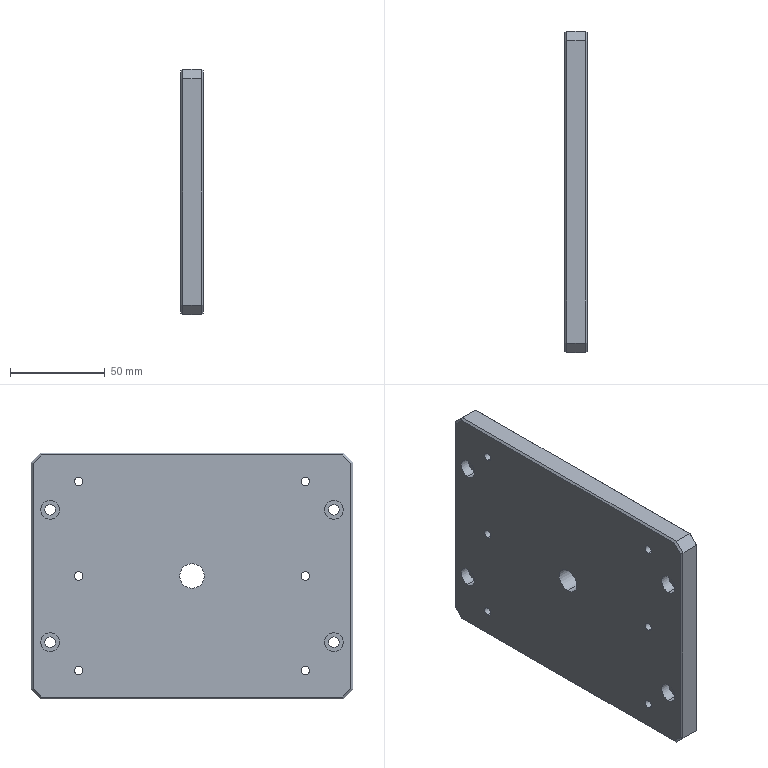Part | STEP file | BPSP-11-18 Unloading Lift Plate_Default | 1 solid | 97 faces | box 12 x 170 x 130 mm | volume 257545 mm3 | cylinder 52 | plane 37 | cone 8 | commonest cylinder face diameters 4.5 x12 7.5 x12 3.3 x8 5.5 x8 10 x8 13 x2